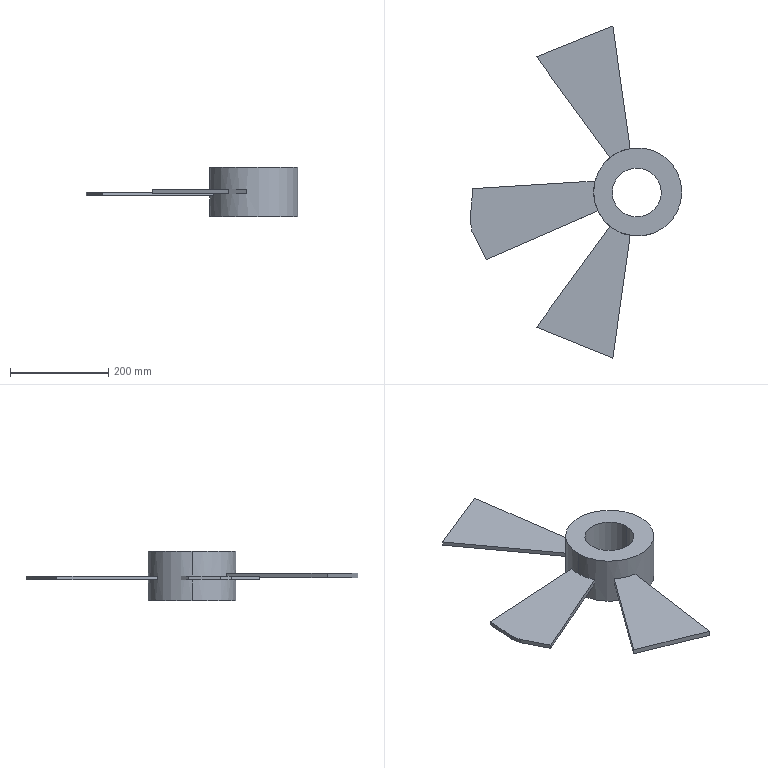Part | SolidWorks | features ICE 4, Extrusion 1 | 1 solid | 23 faces | box 431.967 x 677.234 x 100 mm | volume 2444150 mm3 | plane 19 | cylinder 4 | commonest cylinder face diameters 100 x2 180 x2
STEP:
#1=CARTESIAN_POINT('',(-51.963,-1.128,-46.));
#2=VERTEX_POINT('',#1);
#3=CARTESIAN_POINT('',(48.037,-1.128,-46.));
#4=VERTEX_POINT('',#3);
#5=CARTESIAN_POINT('',(-1.963,-1.128,-46.));
#6=DIRECTION('',(0.,0.,1.));
#7=DIRECTION('',(1.,0.,0.));
#8=AXIS2_PLACEMENT_3D('',#5,#6,#7);
#9=CIRCLE('',#8,50.);
#10=EDGE_CURVE('',#2,#4,#9,.T.);
#11=ORIENTED_EDGE('',*,*,#10,.F.);
#12=CARTESIAN_POINT('',(-51.963,-1.128,54.));
#13=VERTEX_POINT('',#12);
#14=CARTESIAN_POINT('',(-51.963,-1.128,-46.));
#15=DIRECTION('',(0.,0.,1.));
#16=VECTOR('',#15,1000.);
#17=LINE('',#14,#16);
#18=EDGE_CURVE('',#2,#13,#17,.T.);
#19=ORIENTED_EDGE('',*,*,#18,.T.);
#20=CARTESIAN_POINT('',(48.037,-1.128,54.));
#21=VERTEX_POINT('',#20);
#22=CARTESIAN_POINT('',(-1.963,-1.128,54.));
#23=DIRECTION('',(0.,0.,1.));
#24=DIRECTION('',(1.,0.,0.));
#25=AXIS2_PLACEMENT_3D('',#22,#23,#24);
#26=CIRCLE('',#25,50.);
#27=EDGE_CURVE('',#13,#21,#26,.T.);
#28=ORIENTED_EDGE('',*,*,#27,.T.);
#29=CARTESIAN_POINT('',(48.037,-1.128,-46.));
#30=DIRECTION('',(0.,0.,1.));
#31=VECTOR('',#30,1000.);
#32=LINE('',#29,#31);
#33=EDGE_CURVE('',#4,#21,#32,.T.);
#34=ORIENTED_EDGE('',*,*,#33,.F.);
#35=EDGE_LOOP('',(#11,#19,#28,#34));
#36=FACE_OUTER_BOUND('',#35,.T.);
#37=CARTESIAN_POINT('',(-1.963,-1.128,-46.));
#38=DIRECTION('',(0.,0.,1.));
#39=DIRECTION('',(1.,0.,0.));
#40=AXIS2_PLACEMENT_3D('',#37,#38,#39);
#41=CYLINDRICAL_SURFACE('',#40,50.);
#42=ADVANCED_FACE('',(#36),#41,.F.);
#43=CARTESIAN_POINT('',(-15.559,88.645,4.));
#44=VERTEX_POINT('',#43);
#45=CARTESIAN_POINT('',(-15.559,88.645,-4.));
#46=VERTEX_POINT('',#45);
#47=CARTESIAN_POINT('',(-15.559,88.645,54.));
#48=DIRECTION('',(0.,0.,-1.));
#49=VECTOR('',#48,1000.);
#50=LINE('',#47,#49);
#51=EDGE_CURVE('',#44,#46,#50,.T.);
#52=ORIENTED_EDGE('',*,*,#51,.F.);
#53=CARTESIAN_POINT('',(-56.837,69.782,4.));
#54=VERTEX_POINT('',#53);
#55=CARTESIAN_POINT('',(0.,0.,4.));
#56=DIRECTION('',(0.,0.,1.));
#57=DIRECTION('',(1.,0.,0.));
#58=AXIS2_PLACEMENT_3D('',#55,#56,#57);
#59=CIRCLE('',#58,90.);
#60=EDGE_CURVE('',#44,#54,#59,.T.);
#61=ORIENTED_EDGE('',*,*,#60,.T.);
#62=CARTESIAN_POINT('',(-56.837,69.782,-4.));
#63=VERTEX_POINT('',#62);
#64=CARTESIAN_POINT('',(-56.837,69.782,54.));
#65=DIRECTION('',(0.,0.,1.));
#66=VECTOR('',#65,1000.);
#67=LINE('',#64,#66);
#68=EDGE_CURVE('',#63,#54,#67,.T.);
#69=ORIENTED_EDGE('',*,*,#68,.F.);
#70=CARTESIAN_POINT('',(0.,0.,-4.));
#71=DIRECTION('',(0.,0.,1.));
#72=DIRECTION('',(1.,0.,0.));
#73=AXIS2_PLACEMENT_3D('',#70,#71,#72);
#74=CIRCLE('',#73,90.);
#75=EDGE_CURVE('',#46,#63,#74,.T.);
#76=ORIENTED_EDGE('',*,*,#75,.F.);
#77=EDGE_LOOP('',(#52,#61,#69,#76));
#78=FACE_BOUND('',#77,.T.);
#79=CARTESIAN_POINT('',(90.,0.,54.));
#80=VERTEX_POINT('',#79);
#81=CARTESIAN_POINT('',(-90.,0.,54.));
#82=VERTEX_POINT('',#81);
#83=CARTESIAN_POINT('',(0.,0.,54.));
#84=DIRECTION('',(0.,0.,1.));
#85=DIRECTION('',(1.,0.,0.));
#86=AXIS2_PLACEMENT_3D('',#83,#84,#85);
#87=CIRCLE('',#86,90.);
#88=EDGE_CURVE('',#80,#82,#87,.T.);
#89=ORIENTED_EDGE('',*,*,#88,.F.);
#90=CARTESIAN_POINT('',(90.,0.,-46.));
#91=VERTEX_POINT('',#90);
#92=CARTESIAN_POINT('',(90.,0.,54.));
#93=DIRECTION('',(0.,0.,-1.));
#94=VECTOR('',#93,1000.);
#95=LINE('',#92,#94);
#96=EDGE_CURVE('',#80,#91,#95,.T.);
#97=ORIENTED_EDGE('',*,*,#96,.T.);
#98=CARTESIAN_POINT('',(-90.,0.,-46.));
#99=VERTEX_POINT('',#98);
#100=CARTESIAN_POINT('',(0.,0.,-46.));
#101=DIRECTION('',(0.,0.,1.));
#102=DIRECTION('',(1.,0.,0.));
#103=AXIS2_PLACEMENT_3D('',#100,#101,#102);
#104=CIRCLE('',#103,90.);
#105=EDGE_CURVE('',#91,#99,#104,.T.);
#106=ORIENTED_EDGE('',*,*,#105,.T.);
#107=CARTESIAN_POINT('',(-90.,0.,-4.));
#108=VERTEX_POINT('',#107);
#109=CARTESIAN_POINT('',(-90.,0.,54.));
#110=DIRECTION('',(0.,0.,-1.));
#111=VECTOR('',#110,1000.);
#112=LINE('',#109,#111);
#113=EDGE_CURVE('',#108,#99,#112,.T.);
#114=ORIENTED_EDGE('',*,*,#113,.F.);
#115=CARTESIAN_POINT('',(-87.194,22.3,-4.));
#116=VERTEX_POINT('',#115);
#117=CARTESIAN_POINT('',(0.,0.,-4.));
#118=DIRECTION('',(0.,0.,-1.));
#119=DIRECTION('',(1.,0.,0.));
#120=AXIS2_PLACEMENT_3D('',#117,#118,#119);
#121=CIRCLE('',#120,90.);
#122=EDGE_CURVE('',#108,#116,#121,.T.);
#123=ORIENTED_EDGE('',*,*,#122,.T.);
#124=CARTESIAN_POINT('',(-87.194,22.3,4.));
#125=VERTEX_POINT('',#124);
#126=CARTESIAN_POINT('',(-87.194,22.3,54.));
#127=DIRECTION('',(0.,0.,1.));
#128=VECTOR('',#127,1000.);
#129=LINE('',#126,#128);
#130=EDGE_CURVE('',#116,#125,#129,.T.);
#131=ORIENTED_EDGE('',*,*,#130,.T.);
#132=CARTESIAN_POINT('',(-90.,0.,4.));
#133=VERTEX_POINT('',#132);
#134=CARTESIAN_POINT('',(0.,0.,4.));
#135=DIRECTION('',(0.,0.,-1.));
#136=DIRECTION('',(1.,0.,0.));
#137=AXIS2_PLACEMENT_3D('',#134,#135,#136);
#138=CIRCLE('',#137,90.);
#139=EDGE_CURVE('',#133,#125,#138,.T.);
#140=ORIENTED_EDGE('',*,*,#139,.F.);
#141=CARTESIAN_POINT('',(-90.,0.,54.));
#142=DIRECTION('',(0.,0.,-1.));
#143=VECTOR('',#142,1000.);
#144=LINE('',#141,#143);
#145=EDGE_CURVE('',#82,#133,#144,.T.);
#146=ORIENTED_EDGE('',*,*,#145,.F.);
#147=EDGE_LOOP('',(#89,#97,#106,#114,#123,#131,#140,#146));
#148=FACE_OUTER_BOUND('',#147,.T.);
#149=CARTESIAN_POINT('',(0.,0.,54.));
#150=DIRECTION('',(0.,0.,-1.));
#151=DIRECTION('',(-1.,0.,0.));
#152=AXIS2_PLACEMENT_3D('',#149,#150,#151);
#153=CYLINDRICAL_SURFACE('',#152,90.);
#154=ADVANCED_FACE('',(#78,#148),#153,.T.);
#155=ORIENTED_EDGE('',*,*,#96,.F.);
#156=CARTESIAN_POINT('',(0.,0.,54.));
#157=DIRECTION('',(0.,0.,1.));
#158=DIRECTION('',(1.,0.,0.));
#159=AXIS2_PLACEMENT_3D('',#156,#157,#158);
#160=CIRCLE('',#159,90.);
#161=EDGE_CURVE('',#82,#80,#160,.T.);
#162=ORIENTED_EDGE('',*,*,#161,.F.);
#163=ORIENTED_EDGE('',*,*,#145,.T.);
#164=CARTESIAN_POINT('',(-81.236,-38.739,4.));
#165=VERTEX_POINT('',#164);
#166=CARTESIAN_POINT('',(0.,0.,4.));
#167=DIRECTION('',(0.,0.,-1.));
#168=DIRECTION('',(1.,0.,0.));
#169=AXIS2_PLACEMENT_3D('',#166,#167,#168);
#170=CIRCLE('',#169,90.);
#171=EDGE_CURVE('',#165,#133,#170,.T.);
#172=ORIENTED_EDGE('',*,*,#171,.F.);
#173=CARTESIAN_POINT('',(-81.236,-38.739,-4.));
#174=VERTEX_POINT('',#173);
#175=CARTESIAN_POINT('',(-81.236,-38.739,54.));
#176=DIRECTION('',(0.,0.,-1.));
#177=VECTOR('',#176,1000.);
#178=LINE('',#175,#177);
#179=EDGE_CURVE('',#165,#174,#178,.T.);
#180=ORIENTED_EDGE('',*,*,#179,.T.);
#181=CARTESIAN_POINT('',(0.,0.,-4.));
#182=DIRECTION('',(0.,0.,-1.));
#183=DIRECTION('',(1.,0.,0.));
#184=AXIS2_PLACEMENT_3D('',#181,#182,#183);
#185=CIRCLE('',#184,90.);
#186=EDGE_CURVE('',#174,#108,#185,.T.);
#187=ORIENTED_EDGE('',*,*,#186,.T.);
#188=ORIENTED_EDGE('',*,*,#113,.T.);
#189=CARTESIAN_POINT('',(0.,0.,-46.));
#190=DIRECTION('',(0.,0.,1.));
#191=DIRECTION('',(1.,0.,0.));
#192=AXIS2_PLACEMENT_3D('',#189,#190,#191);
#193=CIRCLE('',#192,90.);
#194=EDGE_CURVE('',#99,#91,#193,.T.);
#195=ORIENTED_EDGE('',*,*,#194,.T.);
#196=EDGE_LOOP('',(#155,#162,#163,#172,#180,#187,#188,#195));
#197=FACE_OUTER_BOUND('',#196,.T.);
#198=CARTESIAN_POINT('',(-15.559,-88.645,10.));
#199=VERTEX_POINT('',#198);
#200=CARTESIAN_POINT('',(-56.837,-69.782,10.));
#201=VERTEX_POINT('',#200);
#202=CARTESIAN_POINT('',(0.,0.,10.));
#203=DIRECTION('',(0.,0.,-1.));
#204=DIRECTION('',(-1.,0.,0.));
#205=AXIS2_PLACEMENT_3D('',#202,#203,#204);
#206=CIRCLE('',#205,90.);
#207=EDGE_CURVE('',#199,#201,#206,.T.);
#208=ORIENTED_EDGE('',*,*,#207,.F.);
#209=CARTESIAN_POINT('',(-15.559,-88.645,0.));
#210=VERTEX_POINT('',#209);
#211=CARTESIAN_POINT('',(-15.559,-88.645,10.));
#212=DIRECTION('',(0.,0.,-1.));
#213=VECTOR('',#212,1000.);
#214=LINE('',#211,#213);
#215=EDGE_CURVE('',#199,#210,#214,.T.);
#216=ORIENTED_EDGE('',*,*,#215,.T.);
#217=CARTESIAN_POINT('',(-56.837,-69.782,0.));
#218=VERTEX_POINT('',#217);
#219=CARTESIAN_POINT('',(0.,0.,0.));
#220=DIRECTION('',(0.,0.,-1.));
#221=DIRECTION('',(-1.,0.,0.));
#222=AXIS2_PLACEMENT_3D('',#219,#220,#221);
#223=CIRCLE('',#222,90.);
#224=EDGE_CURVE('',#210,#218,#223,.T.);
#225=ORIENTED_EDGE('',*,*,#224,.T.);
#226=CARTESIAN_POINT('',(-56.837,-69.782,10.));
#227=DIRECTION('',(0.,0.,-1.));
#228=VECTOR('',#227,1000.);
#229=LINE('',#226,#228);
#230=EDGE_CURVE('',#201,#218,#229,.T.);
#231=ORIENTED_EDGE('',*,*,#230,.F.);
#232=EDGE_LOOP('',(#208,#216,#225,#231));
#233=FACE_BOUND('',#232,.T.);
#234=CARTESIAN_POINT('',(0.,0.,54.));
#235=DIRECTION('',(0.,0.,-1.));
#236=DIRECTION('',(-1.,0.,0.));
#237=AXIS2_PLACEMENT_3D('',#234,#235,#236);
#238=CYLINDRICAL_SURFACE('',#237,90.);
#239=ADVANCED_FACE('',(#197,#233),#238,.T.);
#240=ORIENTED_EDGE('',*,*,#130,.F.);
#241=CARTESIAN_POINT('',(-336.508,6.839,-4.));
#242=VERTEX_POINT('',#241);
#243=CARTESIAN_POINT('',(-53.49,24.39,-4.));
#244=DIRECTION('',(-0.9981,-0.06189,0.));
#245=VECTOR('',#244,1000.);
#246=LINE('',#243,#245);
#247=EDGE_CURVE('',#116,#242,#246,.T.);
#248=ORIENTED_EDGE('',*,*,#247,.T.);
#249=CARTESIAN_POINT('',(-336.508,6.839,4.));
#250=VERTEX_POINT('',#249);
#251=CARTESIAN_POINT('',(-336.508,6.839,4.));
#252=DIRECTION('',(0.,0.,-1.));
#253=VECTOR('',#252,1000.);
#254=LINE('',#251,#253);
#255=EDGE_CURVE('',#250,#242,#254,.T.);
#256=ORIENTED_EDGE('',*,*,#255,.F.);
#257=CARTESIAN_POINT('',(-53.49,24.39,4.));
#258=DIRECTION('',(-0.9981,-0.06189,0.));
#259=VECTOR('',#258,1000.);
#260=LINE('',#257,#259);
#261=EDGE_CURVE('',#125,#250,#260,.T.);
#262=ORIENTED_EDGE('',*,*,#261,.F.);
#263=EDGE_LOOP('',(#240,#248,#256,#262));
#264=FACE_OUTER_BOUND('',#263,.T.);
#265=CARTESIAN_POINT('',(-53.49,24.39,4.));
#266=DIRECTION('',(0.06189,-0.9981,0.));
#267=DIRECTION('',(0.9981,0.06189,0.));
#268=AXIS2_PLACEMENT_3D('',#265,#266,#267);
#269=PLANE('',#268);
#270=ADVANCED_FACE('',(#264),#269,.F.);
#271=ORIENTED_EDGE('',*,*,#179,.F.);
#272=CARTESIAN_POINT('',(-308.839,-137.933,4.));
#273=VERTEX_POINT('',#272);
#274=CARTESIAN_POINT('',(-308.839,-137.933,4.));
#275=DIRECTION('',(0.9167,0.3995,0.));
#276=VECTOR('',#275,1000.);
#277=LINE('',#274,#276);
#278=EDGE_CURVE('',#273,#165,#277,.T.);
#279=ORIENTED_EDGE('',*,*,#278,.F.);
#280=CARTESIAN_POINT('',(-308.839,-137.933,-4.));
#281=VERTEX_POINT('',#280);
#282=CARTESIAN_POINT('',(-308.839,-137.933,4.));
#283=DIRECTION('',(0.,0.,-1.));
#284=VECTOR('',#283,1000.);
#285=LINE('',#282,#284);
#286=EDGE_CURVE('',#273,#281,#285,.T.);
#287=ORIENTED_EDGE('',*,*,#286,.T.);
#288=CARTESIAN_POINT('',(-308.839,-137.933,-4.));
#289=DIRECTION('',(0.9167,0.3995,0.));
#290=VECTOR('',#289,1000.);
#291=LINE('',#288,#290);
#292=EDGE_CURVE('',#281,#174,#291,.T.);
#293=ORIENTED_EDGE('',*,*,#292,.T.);
#294=EDGE_LOOP('',(#271,#279,#287,#293));
#295=FACE_OUTER_BOUND('',#294,.T.);
#296=CARTESIAN_POINT('',(-308.839,-137.933,4.));
#297=DIRECTION('',(-0.3995,0.9167,0.));
#298=DIRECTION('',(-0.9167,-0.3995,0.));
#299=AXIS2_PLACEMENT_3D('',#296,#297,#298);
#300=PLANE('',#299);
#301=ADVANCED_FACE('',(#295),#300,.F.);
#302=ORIENTED_EDGE('',*,*,#278,.T.);
#303=ORIENTED_EDGE('',*,*,#171,.T.);
#304=ORIENTED_EDGE('',*,*,#139,.T.);
#305=ORIENTED_EDGE('',*,*,#261,.T.);
#306=CARTESIAN_POINT('',(-341.967,-58.161,4.));
#307=VERTEX_POINT('',#306);
#308=CARTESIAN_POINT('',(-341.967,-58.161,4.));
#309=DIRECTION('',(-0.08368,-0.9965,0.));
#310=VECTOR('',#309,1000.);
#311=LINE('',#308,#310);
#312=EDGE_CURVE('',#250,#307,#311,.T.);
#313=ORIENTED_EDGE('',*,*,#312,.T.);
#314=CARTESIAN_POINT('',(-338.146,-79.915,4.));
#315=VERTEX_POINT('',#314);
#316=CARTESIAN_POINT('',(-341.967,-58.161,4.));
#317=DIRECTION('',(0.173,-0.9849,0.));
#318=VECTOR('',#317,1000.);
#319=LINE('',#316,#318);
#320=EDGE_CURVE('',#307,#315,#319,.T.);
#321=ORIENTED_EDGE('',*,*,#320,.T.);
#322=CARTESIAN_POINT('',(-338.146,-79.915,4.));
#323=DIRECTION('',(0.4509,-0.8926,0.));
#324=VECTOR('',#323,1000.);
#325=LINE('',#322,#324);
#326=EDGE_CURVE('',#315,#273,#325,.T.);
#327=ORIENTED_EDGE('',*,*,#326,.T.);
#328=EDGE_LOOP('',(#302,#303,#304,#305,#313,#321,#327));
#329=FACE_OUTER_BOUND('',#328,.T.);
#330=CARTESIAN_POINT('',(-1.963,-1.128,4.));
#331=DIRECTION('',(0.,0.,1.));
#332=DIRECTION('',(1.,0.,0.));
#333=AXIS2_PLACEMENT_3D('',#330,#331,#332);
#334=PLANE('',#333);
#335=ADVANCED_FACE('',(#329),#334,.T.);
#336=ORIENTED_EDGE('',*,*,#186,.F.);
#337=ORIENTED_EDGE('',*,*,#292,.F.);
#338=CARTESIAN_POINT('',(-338.146,-79.915,-4.));
#339=VERTEX_POINT('',#338);
#340=CARTESIAN_POINT('',(-338.146,-79.915,-4.));
#341=DIRECTION('',(0.4509,-0.8926,0.));
#342=VECTOR('',#341,1000.);
#343=LINE('',#340,#342);
#344=EDGE_CURVE('',#339,#281,#343,.T.);
#345=ORIENTED_EDGE('',*,*,#344,.F.);
#346=CARTESIAN_POINT('',(-341.967,-58.161,-4.));
#347=VERTEX_POINT('',#346);
#348=CARTESIAN_POINT('',(-341.967,-58.161,-4.));
#349=DIRECTION('',(0.173,-0.9849,0.));
#350=VECTOR('',#349,1000.);
#351=LINE('',#348,#350);
#352=EDGE_CURVE('',#347,#339,#351,.T.);
#353=ORIENTED_EDGE('',*,*,#352,.F.);
#354=CARTESIAN_POINT('',(-341.967,-58.161,-4.));
#355=DIRECTION('',(-0.08368,-0.9965,0.));
#356=VECTOR('',#355,1000.);
#357=LINE('',#354,#356);
#358=EDGE_CURVE('',#242,#347,#357,.T.);
#359=ORIENTED_EDGE('',*,*,#358,.F.);
#360=ORIENTED_EDGE('',*,*,#247,.F.);
#361=ORIENTED_EDGE('',*,*,#122,.F.);
#362=EDGE_LOOP('',(#336,#337,#345,#353,#359,#360,#361));
#363=FACE_OUTER_BOUND('',#362,.T.);
#364=CARTESIAN_POINT('',(-1.963,-1.128,-4.));
#365=DIRECTION('',(0.,0.,1.));
#366=DIRECTION('',(1.,0.,0.));
#367=AXIS2_PLACEMENT_3D('',#364,#365,#366);
#368=PLANE('',#367);
#369=ADVANCED_FACE('',(#363),#368,.F.);
#370=ORIENTED_EDGE('',*,*,#358,.T.);
#371=CARTESIAN_POINT('',(-341.967,-58.161,4.));
#372=DIRECTION('',(0.,0.,-1.));
#373=VECTOR('',#372,1000.);
#374=LINE('',#371,#373);
#375=EDGE_CURVE('',#307,#347,#374,.T.);
#376=ORIENTED_EDGE('',*,*,#375,.F.);
#377=ORIENTED_EDGE('',*,*,#312,.F.);
#378=ORIENTED_EDGE('',*,*,#255,.T.);
#379=EDGE_LOOP('',(#370,#376,#377,#378));
#380=FACE_OUTER_BOUND('',#379,.T.);
#381=CARTESIAN_POINT('',(-341.967,-58.161,4.));
#382=DIRECTION('',(0.9965,-0.08368,0.));
#383=DIRECTION('',(0.08368,0.9965,0.));
#384=AXIS2_PLACEMENT_3D('',#381,#382,#383);
#385=PLANE('',#384);
#386=ADVANCED_FACE('',(#380),#385,.F.);
#387=ORIENTED_EDGE('',*,*,#352,.T.);
#388=CARTESIAN_POINT('',(-338.146,-79.915,4.));
#389=DIRECTION('',(0.,0.,-1.));
#390=VECTOR('',#389,1000.);
#391=LINE('',#388,#390);
#392=EDGE_CURVE('',#315,#339,#391,.T.);
#393=ORIENTED_EDGE('',*,*,#392,.F.);
#394=ORIENTED_EDGE('',*,*,#320,.F.);
#395=ORIENTED_EDGE('',*,*,#375,.T.);
#396=EDGE_LOOP('',(#387,#393,#394,#395));
#397=FACE_OUTER_BOUND('',#396,.T.);
#398=CARTESIAN_POINT('',(-341.967,-58.161,4.));
#399=DIRECTION('',(0.9849,0.173,0.));
#400=DIRECTION('',(-0.173,0.9849,0.));
#401=AXIS2_PLACEMENT_3D('',#398,#399,#400);
#402=PLANE('',#401);
#403=ADVANCED_FACE('',(#397),#402,.F.);
#404=ORIENTED_EDGE('',*,*,#344,.T.);
#405=ORIENTED_EDGE('',*,*,#286,.F.);
#406=ORIENTED_EDGE('',*,*,#326,.F.);
#407=ORIENTED_EDGE('',*,*,#392,.T.);
#408=EDGE_LOOP('',(#404,#405,#406,#407));
#409=FACE_OUTER_BOUND('',#408,.T.);
#410=CARTESIAN_POINT('',(-338.146,-79.915,4.));
#411=DIRECTION('',(0.8926,0.4509,0.));
#412=DIRECTION('',(-0.4509,0.8926,0.));
#413=AXIS2_PLACEMENT_3D('',#410,#411,#412);
#414=PLANE('',#413);
#415=ADVANCED_FACE('',(#409),#414,.F.);
#416=ORIENTED_EDGE('',*,*,#161,.T.);
#417=ORIENTED_EDGE('',*,*,#88,.T.);
#418=EDGE_LOOP('',(#416,#417));
#419=FACE_OUTER_BOUND('',#418,.T.);
#420=CARTESIAN_POINT('',(-1.963,-1.128,54.));
#421=DIRECTION('',(0.,0.,1.));
#422=DIRECTION('',(1.,0.,0.));
#423=AXIS2_PLACEMENT_3D('',#420,#421,#422);
#424=CIRCLE('',#423,50.);
#425=EDGE_CURVE('',#21,#13,#424,.T.);
#426=ORIENTED_EDGE('',*,*,#425,.F.);
#427=ORIENTED_EDGE('',*,*,#27,.F.);
#428=EDGE_LOOP('',(#426,#427));
#429=FACE_BOUND('',#428,.T.);
#430=CARTESIAN_POINT('',(0.,0.,54.));
#431=DIRECTION('',(0.,0.,1.));
#432=DIRECTION('',(1.,0.,0.));
#433=AXIS2_PLACEMENT_3D('',#430,#431,#432);
#434=PLANE('',#433);
#435=ADVANCED_FACE('',(#419,#429),#434,.T.);
#436=ORIENTED_EDGE('',*,*,#194,.F.);
#437=ORIENTED_EDGE('',*,*,#105,.F.);
#438=EDGE_LOOP('',(#436,#437));
#439=FACE_OUTER_BOUND('',#438,.T.);
#440=CARTESIAN_POINT('',(-1.963,-1.128,-46.));
#441=DIRECTION('',(0.,0.,1.));
#442=DIRECTION('',(1.,0.,0.));
#443=AXIS2_PLACEMENT_3D('',#440,#441,#442);
#444=CIRCLE('',#443,50.);
#445=EDGE_CURVE('',#4,#2,#444,.T.);
#446=ORIENTED_EDGE('',*,*,#445,.T.);
#447=ORIENTED_EDGE('',*,*,#10,.T.);
#448=EDGE_LOOP('',(#446,#447));
#449=FACE_BOUND('',#448,.T.);
#450=CARTESIAN_POINT('',(0.,0.,-46.));
#451=DIRECTION('',(0.,0.,1.));
#452=DIRECTION('',(1.,0.,0.));
#453=AXIS2_PLACEMENT_3D('',#450,#451,#452);
#454=PLANE('',#453);
#455=ADVANCED_FACE('',(#439,#449),#454,.F.);
#456=CARTESIAN_POINT('',(-206.438,275.691,-4.));
#457=VERTEX_POINT('',#456);
#458=CARTESIAN_POINT('',(-206.438,275.691,-4.));
#459=DIRECTION('',(0.5878,-0.809,0.));
#460=VECTOR('',#459,1000.);
#461=LINE('',#458,#460);
#462=EDGE_CURVE('',#457,#63,#461,.T.);
#463=ORIENTED_EDGE('',*,*,#462,.T.);
#464=ORIENTED_EDGE('',*,*,#68,.T.);
#465=CARTESIAN_POINT('',(-206.438,275.691,4.));
#466=VERTEX_POINT('',#465);
#467=CARTESIAN_POINT('',(-206.438,275.691,4.));
#468=DIRECTION('',(0.5878,-0.809,0.));
#469=VECTOR('',#468,1000.);
#470=LINE('',#467,#469);
#471=EDGE_CURVE('',#466,#54,#470,.T.);
#472=ORIENTED_EDGE('',*,*,#471,.F.);
#473=CARTESIAN_POINT('',(-206.438,275.691,4.));
#474=DIRECTION('',(0.,0.,-1.));
#475=VECTOR('',#474,1000.);
#476=LINE('',#473,#475);
#477=EDGE_CURVE('',#466,#457,#476,.T.);
#478=ORIENTED_EDGE('',*,*,#477,.T.);
#479=EDGE_LOOP('',(#463,#464,#472,#478));
#480=FACE_OUTER_BOUND('',#479,.T.);
#481=CARTESIAN_POINT('',(-206.438,275.691,4.));
#482=DIRECTION('',(0.809,0.5878,0.));
#483=DIRECTION('',(-0.5878,0.809,0.));
#484=AXIS2_PLACEMENT_3D('',#481,#482,#483);
#485=PLANE('',#484);
#486=ADVANCED_FACE('',(#480),#485,.F.);
#487=CARTESIAN_POINT('',(-50.691,338.617,4.));
#488=VERTEX_POINT('',#487);
#489=CARTESIAN_POINT('',(-10.925,55.669,4.));
#490=DIRECTION('',(-0.1392,0.9903,0.));
#491=VECTOR('',#490,1000.);
#492=LINE('',#489,#491);
#493=EDGE_CURVE('',#44,#488,#492,.T.);
#494=ORIENTED_EDGE('',*,*,#493,.F.);
#495=ORIENTED_EDGE('',*,*,#51,.T.);
#496=CARTESIAN_POINT('',(-50.691,338.617,-4.));
#497=VERTEX_POINT('',#496);
#498=CARTESIAN_POINT('',(-10.925,55.669,-4.));
#499=DIRECTION('',(-0.1392,0.9903,0.));
#500=VECTOR('',#499,1000.);
#501=LINE('',#498,#500);
#502=EDGE_CURVE('',#46,#497,#501,.T.);
#503=ORIENTED_EDGE('',*,*,#502,.T.);
#504=CARTESIAN_POINT('',(-50.691,338.617,4.));
#505=DIRECTION('',(0.,0.,-1.));
#506=VECTOR('',#505,1000.);
#507=LINE('',#504,#506);
#508=EDGE_CURVE('',#488,#497,#507,.T.);
#509=ORIENTED_EDGE('',*,*,#508,.F.);
#510=EDGE_LOOP('',(#494,#495,#503,#509));
#511=FACE_OUTER_BOUND('',#510,.T.);
#512=CARTESIAN_POINT('',(-10.925,55.669,4.));
#513=DIRECTION('',(-0.9903,-0.1392,0.));
#514=DIRECTION('',(0.1392,-0.9903,0.));
#515=AXIS2_PLACEMENT_3D('',#512,#513,#514);
#516=PLANE('',#515);
#517=ADVANCED_FACE('',(#511),#516,.F.);
#518=ORIENTED_EDGE('',*,*,#60,.F.);
#519=ORIENTED_EDGE('',*,*,#493,.T.);
#520=CARTESIAN_POINT('',(-50.691,338.617,4.));
#521=DIRECTION('',(-0.9272,-0.3746,0.));
#522=VECTOR('',#521,1000.);
#523=LINE('',#520,#522);
#524=EDGE_CURVE('',#488,#466,#523,.T.);
#525=ORIENTED_EDGE('',*,*,#524,.T.);
#526=ORIENTED_EDGE('',*,*,#471,.T.);
#527=EDGE_LOOP('',(#518,#519,#525,#526));
#528=FACE_OUTER_BOUND('',#527,.T.);
#529=CARTESIAN_POINT('',(-1.963,-1.128,4.));
#530=DIRECTION('',(0.,0.,1.));
#531=DIRECTION('',(1.,0.,0.));
#532=AXIS2_PLACEMENT_3D('',#529,#530,#531);
#533=PLANE('',#532);
#534=ADVANCED_FACE('',(#528),#533,.T.);
#535=ORIENTED_EDGE('',*,*,#502,.F.);
#536=ORIENTED_EDGE('',*,*,#75,.T.);
#537=ORIENTED_EDGE('',*,*,#462,.F.);
#538=CARTESIAN_POINT('',(-50.691,338.617,-4.));
#539=DIRECTION('',(-0.9272,-0.3746,0.));
#540=VECTOR('',#539,1000.);
#541=LINE('',#538,#540);
#542=EDGE_CURVE('',#497,#457,#541,.T.);
#543=ORIENTED_EDGE('',*,*,#542,.F.);
#544=EDGE_LOOP('',(#535,#536,#537,#543));
#545=FACE_OUTER_BOUND('',#544,.T.);
#546=CARTESIAN_POINT('',(-1.963,-1.128,-4.));
#547=DIRECTION('',(0.,0.,1.));
#548=DIRECTION('',(1.,0.,0.));
#549=AXIS2_PLACEMENT_3D('',#546,#547,#548);
#550=PLANE('',#549);
#551=ADVANCED_FACE('',(#545),#550,.F.);
#552=ORIENTED_EDGE('',*,*,#542,.T.);
#553=ORIENTED_EDGE('',*,*,#477,.F.);
#554=ORIENTED_EDGE('',*,*,#524,.F.);
#555=ORIENTED_EDGE('',*,*,#508,.T.);
#556=EDGE_LOOP('',(#552,#553,#554,#555));
#557=FACE_OUTER_BOUND('',#556,.T.);
#558=CARTESIAN_POINT('',(-50.691,338.617,4.));
#559=DIRECTION('',(0.3746,-0.9272,0.));
#560=DIRECTION('',(0.9272,0.3746,0.));
#561=AXIS2_PLACEMENT_3D('',#558,#559,#560);
#562=PLANE('',#561);
#563=ADVANCED_FACE('',(#557),#562,.F.);
#564=ORIENTED_EDGE('',*,*,#18,.F.);
#565=ORIENTED_EDGE('',*,*,#445,.F.);
#566=ORIENTED_EDGE('',*,*,#33,.T.);
#567=ORIENTED_EDGE('',*,*,#425,.T.);
#568=EDGE_LOOP('',(#564,#565,#566,#567));
#569=FACE_OUTER_BOUND('',#568,.T.);
#570=CARTESIAN_POINT('',(-1.963,-1.128,-46.));
#571=DIRECTION('',(0.,0.,1.));
#572=DIRECTION('',(1.,0.,0.));
#573=AXIS2_PLACEMENT_3D('',#570,#571,#572);
#574=CYLINDRICAL_SURFACE('',#573,50.);
#575=ADVANCED_FACE('',(#569),#574,.F.);
#576=CARTESIAN_POINT('',(-206.438,-275.691,0.));
#577=VERTEX_POINT('',#576);
#578=CARTESIAN_POINT('',(-206.438,-275.691,0.));
#579=DIRECTION('',(0.5878,0.809,0.));
#580=VECTOR('',#579,1000.);
#581=LINE('',#578,#580);
#582=EDGE_CURVE('',#577,#218,#581,.T.);
#583=ORIENTED_EDGE('',*,*,#582,.F.);
#584=CARTESIAN_POINT('',(-206.438,-275.691,10.));
#585=VERTEX_POINT('',#584);
#586=CARTESIAN_POINT('',(-206.438,-275.691,10.));
#587=DIRECTION('',(0.,0.,-1.));
#588=VECTOR('',#587,1000.);
#589=LINE('',#586,#588);
#590=EDGE_CURVE('',#585,#577,#589,.T.);
#591=ORIENTED_EDGE('',*,*,#590,.F.);
#592=CARTESIAN_POINT('',(-206.438,-275.691,10.));
#593=DIRECTION('',(0.5878,0.809,0.));
#594=VECTOR('',#593,1000.);
#595=LINE('',#592,#594);
#596=EDGE_CURVE('',#585,#201,#595,.T.);
#597=ORIENTED_EDGE('',*,*,#596,.T.);
#598=ORIENTED_EDGE('',*,*,#230,.T.);
#599=EDGE_LOOP('',(#583,#591,#597,#598));
#600=FACE_OUTER_BOUND('',#599,.T.);
#601=CARTESIAN_POINT('',(-206.438,-275.691,10.));
#602=DIRECTION('',(-0.809,0.5878,0.));
#603=DIRECTION('',(-0.5878,-0.809,0.));
#604=AXIS2_PLACEMENT_3D('',#601,#602,#603);
#605=PLANE('',#604);
#606=ADVANCED_FACE('',(#600),#605,.T.);
#607=CARTESIAN_POINT('',(-50.691,-338.617,0.));
#608=VERTEX_POINT('',#607);
#609=CARTESIAN_POINT('',(-50.691,-338.617,0.));
#610=DIRECTION('',(-0.9272,0.3746,0.));
#611=VECTOR('',#610,1000.);
#612=LINE('',#609,#611);
#613=EDGE_CURVE('',#608,#577,#612,.T.);
#614=ORIENTED_EDGE('',*,*,#613,.F.);
#615=CARTESIAN_POINT('',(-50.691,-338.617,10.));
#616=VERTEX_POINT('',#615);
#617=CARTESIAN_POINT('',(-50.691,-338.617,10.));
#618=DIRECTION('',(0.,0.,-1.));
#619=VECTOR('',#618,1000.);
#620=LINE('',#617,#619);
#621=EDGE_CURVE('',#616,#608,#620,.T.);
#622=ORIENTED_EDGE('',*,*,#621,.F.);
#623=CARTESIAN_POINT('',(-50.691,-338.617,10.));
#624=DIRECTION('',(-0.9272,0.3746,0.));
#625=VECTOR('',#624,1000.);
#626=LINE('',#623,#625);
#627=EDGE_CURVE('',#616,#585,#626,.T.);
#628=ORIENTED_EDGE('',*,*,#627,.T.);
#629=ORIENTED_EDGE('',*,*,#590,.T.);
#630=EDGE_LOOP('',(#614,#622,#628,#629));
#631=FACE_OUTER_BOUND('',#630,.T.);
#632=CARTESIAN_POINT('',(-50.691,-338.617,10.));
#633=DIRECTION('',(-0.3746,-0.9272,0.));
#634=DIRECTION('',(0.9272,-0.3746,0.));
#635=AXIS2_PLACEMENT_3D('',#632,#633,#634);
#636=PLANE('',#635);
#637=ADVANCED_FACE('',(#631),#636,.T.);
#638=CARTESIAN_POINT('',(-15.559,-88.645,0.));
#639=DIRECTION('',(-0.1392,-0.9903,0.));
#640=VECTOR('',#639,1000.);
#641=LINE('',#638,#640);
#642=EDGE_CURVE('',#210,#608,#641,.T.);
#643=ORIENTED_EDGE('',*,*,#642,.F.);
#644=ORIENTED_EDGE('',*,*,#215,.F.);
#645=CARTESIAN_POINT('',(-15.559,-88.645,10.));
#646=DIRECTION('',(-0.1392,-0.9903,0.));
#647=VECTOR('',#646,1000.);
#648=LINE('',#645,#647);
#649=EDGE_CURVE('',#199,#616,#648,.T.);
#650=ORIENTED_EDGE('',*,*,#649,.T.);
#651=ORIENTED_EDGE('',*,*,#621,.T.);
#652=EDGE_LOOP('',(#643,#644,#650,#651));
#653=FACE_OUTER_BOUND('',#652,.T.);
#654=CARTESIAN_POINT('',(-15.559,-88.645,10.));
#655=DIRECTION('',(0.9903,-0.1392,0.));
#656=DIRECTION('',(0.1392,0.9903,0.));
#657=AXIS2_PLACEMENT_3D('',#654,#655,#656);
#658=PLANE('',#657);
#659=ADVANCED_FACE('',(#653),#658,.T.);
#660=ORIENTED_EDGE('',*,*,#207,.T.);
#661=ORIENTED_EDGE('',*,*,#596,.F.);
#662=ORIENTED_EDGE('',*,*,#627,.F.);
#663=ORIENTED_EDGE('',*,*,#649,.F.);
#664=EDGE_LOOP('',(#660,#661,#662,#663));
#665=FACE_OUTER_BOUND('',#664,.T.);
#666=CARTESIAN_POINT('',(0.,0.,10.));
#667=DIRECTION('',(0.,0.,-1.));
#668=DIRECTION('',(-1.,0.,0.));
#669=AXIS2_PLACEMENT_3D('',#666,#667,#668);
#670=PLANE('',#669);
#671=ADVANCED_FACE('',(#665),#670,.F.);
#672=ORIENTED_EDGE('',*,*,#224,.F.);
#673=ORIENTED_EDGE('',*,*,#642,.T.);
#674=ORIENTED_EDGE('',*,*,#613,.T.);
#675=ORIENTED_EDGE('',*,*,#582,.T.);
#676=EDGE_LOOP('',(#672,#673,#674,#675));
#677=FACE_OUTER_BOUND('',#676,.T.);
#678=CARTESIAN_POINT('',(0.,0.,0.));
#679=DIRECTION('',(0.,0.,-1.));
#680=DIRECTION('',(-1.,0.,0.));
#681=AXIS2_PLACEMENT_3D('',#678,#679,#680);
#682=PLANE('',#681);
#683=ADVANCED_FACE('',(#677),#682,.T.);
#684=CLOSED_SHELL('',(#42,#154,#239,#270,#301,#335,#369,#386,#403,#415,#435,#455,#486,#517,#534,#551,#563,#575,#606,#637,#659,#671,#683));
#685=MANIFOLD_SOLID_BREP('',#684);
#686=CARTESIAN_POINT('',(0.,0.,0.));
#687=DIRECTION('',(0.,0.,1.));
#688=DIRECTION('',(1.,0.,0.));
#689=AXIS2_PLACEMENT_3D('',#686,#687,#688);
#690=(LENGTH_UNIT()NAMED_UNIT(*)SI_UNIT(.MILLI.,.METRE.));
#691=UNCERTAINTY_MEASURE_WITH_UNIT(LENGTH_MEASURE(0.00001),#690,'','');
#692=(NAMED_UNIT(*)PLANE_ANGLE_UNIT()SI_UNIT($,.RADIAN.));
#693=(NAMED_UNIT(*)SI_UNIT($,.STERADIAN.)SOLID_ANGLE_UNIT());
#694=(GEOMETRIC_REPRESENTATION_CONTEXT(3)GLOBAL_UNCERTAINTY_ASSIGNED_CONTEXT((#691))GLOBAL_UNIT_ASSIGNED_CONTEXT((#690,#692,#693))REPRESENTATION_CONTEXT('',''));
#695=ADVANCED_BREP_SHAPE_REPRESENTATION('',(#685,#689),#694);